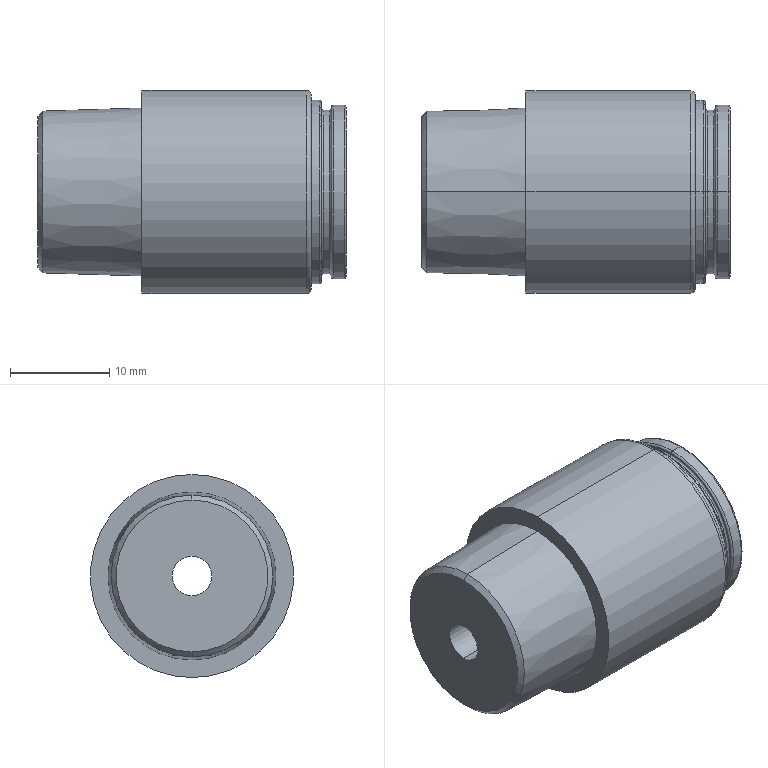Part | STEP file | FITTING-UNION-10AxD12 | 1 solid | 35 faces | box 31.1 x 20.5 x 20.5 mm | volume 6256 mm3 | torus 12 | cylinder 12 | plane 7 | cone 4 | commonest cylinder face diameters 4 x2 12 x2 16.5 x2 17.5 x2 18.5 x2 20.5 x2